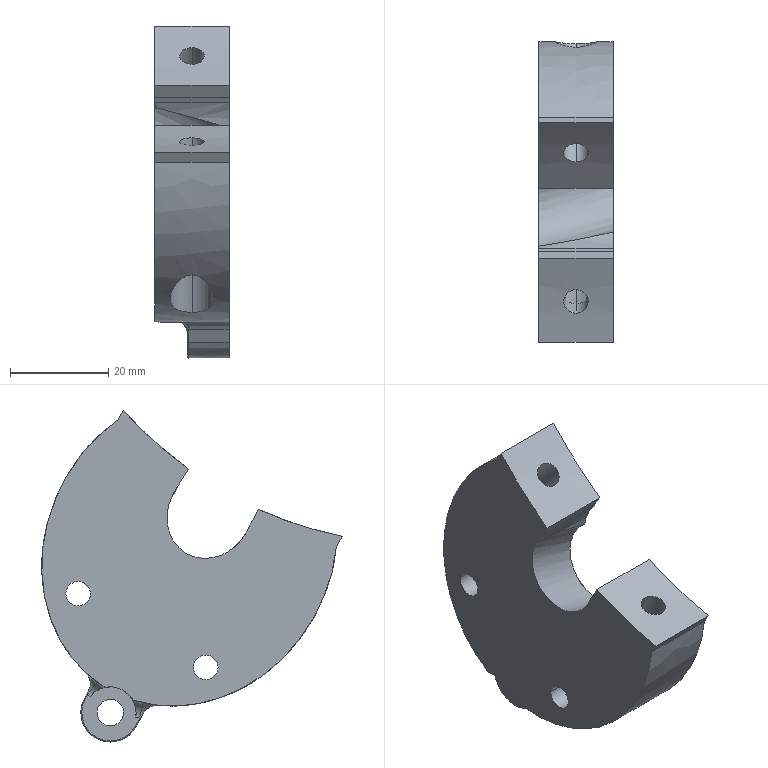Part | STEP file | Completa.sldasm-Part-52_Valor predeterminado | 1 solid | 51 faces | box 15.101 x 61.196 x 67.604 mm | volume 27534 mm3 | cylinder 25 | spline 14 | plane 9 | torus 3 | commonest cylinder face diameters 5 x8 8.9 x4 6.4 x3 0.4 x2 5.4 x2 10.5 x2